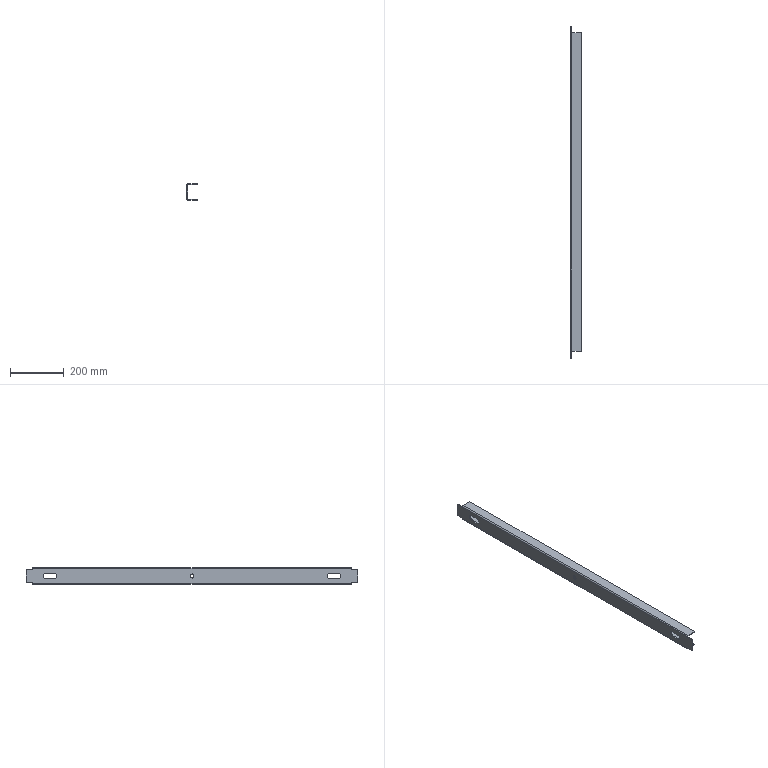Part | SolidWorks | features SMBaseFlange 2, Cut 1, Fillet 1, FlatPattern 1, SheetMetal 1 | 1 solid | 44 faces | box 40 x 1240 x 62 mm | volume 630088 mm3 | plane 30 | cylinder 14 | commonest cylinder face diameters 10 x4 20 x4 0.4 x2 8.4 x2 15 x2
STEP:
#1=CARTESIAN_POINT('',(0.,0.,-7.5));
#2=VERTEX_POINT('',#1);
#3=CARTESIAN_POINT('',(0.,0.,7.5));
#4=VERTEX_POINT('',#3);
#5=CARTESIAN_POINT('',(0.,0.,0.));
#6=DIRECTION('',(-1.,0.,0.));
#7=DIRECTION('',(0.,0.,1.));
#8=AXIS2_PLACEMENT_3D('',#5,#6,#7);
#9=CIRCLE('',#8,7.5);
#10=EDGE_CURVE('',#2,#4,#9,.T.);
#11=ORIENTED_EDGE('',*,*,#10,.T.);
#12=CARTESIAN_POINT('',(4.,0.,7.5));
#13=VERTEX_POINT('',#12);
#14=CARTESIAN_POINT('',(-6.,0.,7.5));
#15=DIRECTION('',(1.,0.,0.));
#16=VECTOR('',#15,1000.);
#17=LINE('',#14,#16);
#18=EDGE_CURVE('',#4,#13,#17,.T.);
#19=ORIENTED_EDGE('',*,*,#18,.T.);
#20=CARTESIAN_POINT('',(4.,0.,-7.5));
#21=VERTEX_POINT('',#20);
#22=CARTESIAN_POINT('',(4.,0.,0.));
#23=DIRECTION('',(1.,0.,0.));
#24=DIRECTION('',(0.,0.,-1.));
#25=AXIS2_PLACEMENT_3D('',#22,#23,#24);
#26=CIRCLE('',#25,7.5);
#27=EDGE_CURVE('',#13,#21,#26,.T.);
#28=ORIENTED_EDGE('',*,*,#27,.T.);
#29=CARTESIAN_POINT('',(-6.,0.,-7.5));
#30=DIRECTION('',(1.,0.,0.));
#31=VECTOR('',#30,1000.);
#32=LINE('',#29,#31);
#33=EDGE_CURVE('',#2,#21,#32,.T.);
#34=ORIENTED_EDGE('',*,*,#33,.F.);
#35=EDGE_LOOP('',(#11,#19,#28,#34));
#36=FACE_OUTER_BOUND('',#35,.T.);
#37=CARTESIAN_POINT('',(-6.,0.,0.));
#38=DIRECTION('',(1.,0.,0.));
#39=DIRECTION('',(0.,0.,-1.));
#40=AXIS2_PLACEMENT_3D('',#37,#38,#39);
#41=CYLINDRICAL_SURFACE('',#40,7.5);
#42=ADVANCED_FACE('',(#36),#41,.F.);
#43=CARTESIAN_POINT('',(4.,-594.,25.));
#44=VERTEX_POINT('',#43);
#45=CARTESIAN_POINT('',(0.,-594.,25.));
#46=VERTEX_POINT('',#45);
#47=CARTESIAN_POINT('',(4.2,-594.,25.));
#48=DIRECTION('',(-1.,0.,0.));
#49=VECTOR('',#48,1000.);
#50=LINE('',#47,#49);
#51=EDGE_CURVE('',#44,#46,#50,.T.);
#52=ORIENTED_EDGE('',*,*,#51,.F.);
#53=CARTESIAN_POINT('',(4.,-594.,26.8));
#54=VERTEX_POINT('',#53);
#55=CARTESIAN_POINT('',(4.,-594.,-31.));
#56=DIRECTION('',(0.,0.,-1.));
#57=VECTOR('',#56,1000.);
#58=LINE('',#55,#57);
#59=EDGE_CURVE('',#54,#44,#58,.T.);
#60=ORIENTED_EDGE('',*,*,#59,.F.);
#61=CARTESIAN_POINT('',(0.,-594.,26.8));
#62=VERTEX_POINT('',#61);
#63=CARTESIAN_POINT('',(4.,-594.,26.8));
#64=DIRECTION('',(-1.,0.,0.));
#65=VECTOR('',#64,1000.);
#66=LINE('',#63,#65);
#67=EDGE_CURVE('',#54,#62,#66,.T.);
#68=ORIENTED_EDGE('',*,*,#67,.T.);
#69=CARTESIAN_POINT('',(0.,-594.,-31.));
#70=DIRECTION('',(0.,0.,-1.));
#71=VECTOR('',#70,1000.);
#72=LINE('',#69,#71);
#73=EDGE_CURVE('',#62,#46,#72,.T.);
#74=ORIENTED_EDGE('',*,*,#73,.T.);
#75=EDGE_LOOP('',(#52,#60,#68,#74));
#76=FACE_OUTER_BOUND('',#75,.T.);
#77=CARTESIAN_POINT('',(4.2,-594.,-27.));
#78=DIRECTION('',(0.,-1.,0.));
#79=DIRECTION('',(0.,0.,-1.));
#80=AXIS2_PLACEMENT_3D('',#77,#78,#79);
#81=PLANE('',#80);
#82=ADVANCED_FACE('',(#76),#81,.T.);
#83=CARTESIAN_POINT('',(4.,594.,-25.));
#84=VERTEX_POINT('',#83);
#85=CARTESIAN_POINT('',(0.,594.,-25.));
#86=VERTEX_POINT('',#85);
#87=CARTESIAN_POINT('',(4.2,594.,-25.));
#88=DIRECTION('',(-1.,0.,0.));
#89=VECTOR('',#88,1000.);
#90=LINE('',#87,#89);
#91=EDGE_CURVE('',#84,#86,#90,.T.);
#92=ORIENTED_EDGE('',*,*,#91,.F.);
#93=CARTESIAN_POINT('',(4.,594.,-26.8));
#94=VERTEX_POINT('',#93);
#95=CARTESIAN_POINT('',(4.,594.,-31.));
#96=DIRECTION('',(0.,0.,-1.));
#97=VECTOR('',#96,1000.);
#98=LINE('',#95,#97);
#99=EDGE_CURVE('',#84,#94,#98,.T.);
#100=ORIENTED_EDGE('',*,*,#99,.T.);
#101=CARTESIAN_POINT('',(0.,594.,-26.8));
#102=VERTEX_POINT('',#101);
#103=CARTESIAN_POINT('',(4.,594.,-26.8));
#104=DIRECTION('',(-1.,0.,0.));
#105=VECTOR('',#104,1000.);
#106=LINE('',#103,#105);
#107=EDGE_CURVE('',#94,#102,#106,.T.);
#108=ORIENTED_EDGE('',*,*,#107,.T.);
#109=CARTESIAN_POINT('',(0.,594.,-31.));
#110=DIRECTION('',(0.,0.,-1.));
#111=VECTOR('',#110,1000.);
#112=LINE('',#109,#111);
#113=EDGE_CURVE('',#86,#102,#112,.T.);
#114=ORIENTED_EDGE('',*,*,#113,.F.);
#115=EDGE_LOOP('',(#92,#100,#108,#114));
#116=FACE_OUTER_BOUND('',#115,.T.);
#117=CARTESIAN_POINT('',(4.2,594.,27.));
#118=DIRECTION('',(0.,1.,0.));
#119=DIRECTION('',(0.,0.,1.));
#120=AXIS2_PLACEMENT_3D('',#117,#118,#119);
#121=PLANE('',#120);
#122=ADVANCED_FACE('',(#116),#121,.T.);
#123=CARTESIAN_POINT('',(0.,594.,26.8));
#124=VERTEX_POINT('',#123);
#125=CARTESIAN_POINT('',(4.,594.,26.8));
#126=VERTEX_POINT('',#125);
#127=CARTESIAN_POINT('',(0.,594.,26.8));
#128=DIRECTION('',(1.,0.,0.));
#129=VECTOR('',#128,1000.);
#130=LINE('',#127,#129);
#131=EDGE_CURVE('',#124,#126,#130,.T.);
#132=ORIENTED_EDGE('',*,*,#131,.F.);
#133=CARTESIAN_POINT('',(4.2,594.,31.));
#134=VERTEX_POINT('',#133);
#135=CARTESIAN_POINT('',(4.2,594.,26.8));
#136=DIRECTION('',(0.,-1.,0.));
#137=DIRECTION('',(0.,0.,1.));
#138=AXIS2_PLACEMENT_3D('',#135,#136,#137);
#139=CIRCLE('',#138,4.2);
#140=EDGE_CURVE('',#134,#124,#139,.T.);
#141=ORIENTED_EDGE('',*,*,#140,.F.);
#142=CARTESIAN_POINT('',(4.2,594.,27.));
#143=VERTEX_POINT('',#142);
#144=CARTESIAN_POINT('',(4.2,594.,27.));
#145=DIRECTION('',(0.,0.,1.));
#146=VECTOR('',#145,1000.);
#147=LINE('',#144,#146);
#148=EDGE_CURVE('',#143,#134,#147,.T.);
#149=ORIENTED_EDGE('',*,*,#148,.F.);
#150=CARTESIAN_POINT('',(4.2,594.,26.8));
#151=DIRECTION('',(0.,-1.,0.));
#152=DIRECTION('',(1.,0.,0.));
#153=AXIS2_PLACEMENT_3D('',#150,#151,#152);
#154=CIRCLE('',#153,0.2);
#155=EDGE_CURVE('',#143,#126,#154,.T.);
#156=ORIENTED_EDGE('',*,*,#155,.T.);
#157=EDGE_LOOP('',(#132,#141,#149,#156));
#158=FACE_OUTER_BOUND('',#157,.T.);
#159=CARTESIAN_POINT('',(0.,594.,26.8));
#160=DIRECTION('',(0.,1.,0.));
#161=DIRECTION('',(0.,0.,1.));
#162=AXIS2_PLACEMENT_3D('',#159,#160,#161);
#163=PLANE('',#162);
#164=ADVANCED_FACE('',(#158),#163,.T.);
#165=CARTESIAN_POINT('',(0.,594.,25.));
#166=VERTEX_POINT('',#165);
#167=CARTESIAN_POINT('',(4.,594.,25.));
#168=VERTEX_POINT('',#167);
#169=CARTESIAN_POINT('',(4.2,594.,25.));
#170=DIRECTION('',(1.,0.,0.));
#171=VECTOR('',#170,1000.);
#172=LINE('',#169,#171);
#173=EDGE_CURVE('',#166,#168,#172,.T.);
#174=ORIENTED_EDGE('',*,*,#173,.F.);
#175=CARTESIAN_POINT('',(0.,594.,-31.));
#176=DIRECTION('',(0.,0.,-1.));
#177=VECTOR('',#176,1000.);
#178=LINE('',#175,#177);
#179=EDGE_CURVE('',#124,#166,#178,.T.);
#180=ORIENTED_EDGE('',*,*,#179,.F.);
#181=ORIENTED_EDGE('',*,*,#131,.T.);
#182=CARTESIAN_POINT('',(4.,594.,-31.));
#183=DIRECTION('',(0.,0.,-1.));
#184=VECTOR('',#183,1000.);
#185=LINE('',#182,#184);
#186=EDGE_CURVE('',#126,#168,#185,.T.);
#187=ORIENTED_EDGE('',*,*,#186,.T.);
#188=EDGE_LOOP('',(#174,#180,#181,#187));
#189=FACE_OUTER_BOUND('',#188,.T.);
#190=CARTESIAN_POINT('',(4.2,594.,27.));
#191=DIRECTION('',(0.,1.,0.));
#192=DIRECTION('',(0.,0.,1.));
#193=AXIS2_PLACEMENT_3D('',#190,#191,#192);
#194=PLANE('',#193);
#195=ADVANCED_FACE('',(#189),#194,.T.);
#196=CARTESIAN_POINT('',(4.2,-594.,31.));
#197=VERTEX_POINT('',#196);
#198=CARTESIAN_POINT('',(4.2,-594.,27.));
#199=VERTEX_POINT('',#198);
#200=CARTESIAN_POINT('',(4.2,-594.,31.));
#201=DIRECTION('',(0.,0.,-1.));
#202=VECTOR('',#201,1000.);
#203=LINE('',#200,#202);
#204=EDGE_CURVE('',#197,#199,#203,.T.);
#205=ORIENTED_EDGE('',*,*,#204,.F.);
#206=CARTESIAN_POINT('',(4.2,-594.,26.8));
#207=DIRECTION('',(0.,-1.,0.));
#208=DIRECTION('',(0.,0.,1.));
#209=AXIS2_PLACEMENT_3D('',#206,#207,#208);
#210=CIRCLE('',#209,4.2);
#211=EDGE_CURVE('',#197,#62,#210,.T.);
#212=ORIENTED_EDGE('',*,*,#211,.T.);
#213=ORIENTED_EDGE('',*,*,#67,.F.);
#214=CARTESIAN_POINT('',(4.2,-594.,26.8));
#215=DIRECTION('',(0.,-1.,0.));
#216=DIRECTION('',(1.,0.,0.));
#217=AXIS2_PLACEMENT_3D('',#214,#215,#216);
#218=CIRCLE('',#217,0.2);
#219=EDGE_CURVE('',#199,#54,#218,.T.);
#220=ORIENTED_EDGE('',*,*,#219,.F.);
#221=EDGE_LOOP('',(#205,#212,#213,#220));
#222=FACE_OUTER_BOUND('',#221,.T.);
#223=CARTESIAN_POINT('',(4.2,-594.,31.));
#224=DIRECTION('',(0.,-1.,0.));
#225=DIRECTION('',(0.,0.,-1.));
#226=AXIS2_PLACEMENT_3D('',#223,#224,#225);
#227=PLANE('',#226);
#228=ADVANCED_FACE('',(#222),#227,.T.);
#229=CARTESIAN_POINT('',(40.,-594.,31.));
#230=VERTEX_POINT('',#229);
#231=CARTESIAN_POINT('',(0.,-594.,31.));
#232=DIRECTION('',(-1.,0.,0.));
#233=VECTOR('',#232,1000.);
#234=LINE('',#231,#233);
#235=EDGE_CURVE('',#230,#197,#234,.T.);
#236=ORIENTED_EDGE('',*,*,#235,.T.);
#237=ORIENTED_EDGE('',*,*,#204,.T.);
#238=CARTESIAN_POINT('',(40.,-594.,27.));
#239=VERTEX_POINT('',#238);
#240=CARTESIAN_POINT('',(0.,-594.,27.));
#241=DIRECTION('',(-1.,0.,0.));
#242=VECTOR('',#241,1000.);
#243=LINE('',#240,#242);
#244=EDGE_CURVE('',#239,#199,#243,.T.);
#245=ORIENTED_EDGE('',*,*,#244,.F.);
#246=CARTESIAN_POINT('',(40.,-594.,27.));
#247=DIRECTION('',(0.,0.,1.));
#248=VECTOR('',#247,1000.);
#249=LINE('',#246,#248);
#250=EDGE_CURVE('',#239,#230,#249,.T.);
#251=ORIENTED_EDGE('',*,*,#250,.T.);
#252=EDGE_LOOP('',(#236,#237,#245,#251));
#253=FACE_OUTER_BOUND('',#252,.T.);
#254=CARTESIAN_POINT('',(4.,-594.,26.8));
#255=DIRECTION('',(0.,-1.,0.));
#256=DIRECTION('',(0.,0.,-1.));
#257=AXIS2_PLACEMENT_3D('',#254,#255,#256);
#258=PLANE('',#257);
#259=ADVANCED_FACE('',(#253),#258,.T.);
#260=CARTESIAN_POINT('',(4.2,594.,-31.));
#261=VERTEX_POINT('',#260);
#262=CARTESIAN_POINT('',(4.2,594.,-27.));
#263=VERTEX_POINT('',#262);
#264=CARTESIAN_POINT('',(4.2,594.,-31.));
#265=DIRECTION('',(0.,0.,1.));
#266=VECTOR('',#265,1000.);
#267=LINE('',#264,#266);
#268=EDGE_CURVE('',#261,#263,#267,.T.);
#269=ORIENTED_EDGE('',*,*,#268,.F.);
#270=CARTESIAN_POINT('',(4.2,594.,-26.8));
#271=DIRECTION('',(0.,-1.,0.));
#272=DIRECTION('',(0.,0.,1.));
#273=AXIS2_PLACEMENT_3D('',#270,#271,#272);
#274=CIRCLE('',#273,4.2);
#275=EDGE_CURVE('',#102,#261,#274,.T.);
#276=ORIENTED_EDGE('',*,*,#275,.F.);
#277=ORIENTED_EDGE('',*,*,#107,.F.);
#278=CARTESIAN_POINT('',(4.2,594.,-26.8));
#279=DIRECTION('',(0.,-1.,0.));
#280=DIRECTION('',(1.,0.,0.));
#281=AXIS2_PLACEMENT_3D('',#278,#279,#280);
#282=CIRCLE('',#281,0.2);
#283=EDGE_CURVE('',#94,#263,#282,.T.);
#284=ORIENTED_EDGE('',*,*,#283,.T.);
#285=EDGE_LOOP('',(#269,#276,#277,#284));
#286=FACE_OUTER_BOUND('',#285,.T.);
#287=CARTESIAN_POINT('',(4.2,594.,-31.));
#288=DIRECTION('',(0.,1.,0.));
#289=DIRECTION('',(0.,0.,1.));
#290=AXIS2_PLACEMENT_3D('',#287,#288,#289);
#291=PLANE('',#290);
#292=ADVANCED_FACE('',(#286),#291,.T.);
#293=CARTESIAN_POINT('',(40.,594.,-31.));
#294=VERTEX_POINT('',#293);
#295=CARTESIAN_POINT('',(0.,594.,-31.));
#296=DIRECTION('',(1.,0.,0.));
#297=VECTOR('',#296,1000.);
#298=LINE('',#295,#297);
#299=EDGE_CURVE('',#261,#294,#298,.T.);
#300=ORIENTED_EDGE('',*,*,#299,.F.);
#301=ORIENTED_EDGE('',*,*,#268,.T.);
#302=CARTESIAN_POINT('',(40.,594.,-27.));
#303=VERTEX_POINT('',#302);
#304=CARTESIAN_POINT('',(0.,594.,-27.));
#305=DIRECTION('',(1.,0.,0.));
#306=VECTOR('',#305,1000.);
#307=LINE('',#304,#306);
#308=EDGE_CURVE('',#263,#303,#307,.T.);
#309=ORIENTED_EDGE('',*,*,#308,.T.);
#310=CARTESIAN_POINT('',(40.,594.,-31.));
#311=DIRECTION('',(0.,0.,1.));
#312=VECTOR('',#311,1000.);
#313=LINE('',#310,#312);
#314=EDGE_CURVE('',#294,#303,#313,.T.);
#315=ORIENTED_EDGE('',*,*,#314,.F.);
#316=EDGE_LOOP('',(#300,#301,#309,#315));
#317=FACE_OUTER_BOUND('',#316,.T.);
#318=CARTESIAN_POINT('',(4.,594.,-26.8));
#319=DIRECTION('',(0.,1.,0.));
#320=DIRECTION('',(0.,0.,1.));
#321=AXIS2_PLACEMENT_3D('',#318,#319,#320);
#322=PLANE('',#321);
#323=ADVANCED_FACE('',(#317),#322,.T.);
#324=CARTESIAN_POINT('',(0.,-594.,-26.8));
#325=VERTEX_POINT('',#324);
#326=CARTESIAN_POINT('',(4.,-594.,-26.8));
#327=VERTEX_POINT('',#326);
#328=CARTESIAN_POINT('',(0.,-594.,-26.8));
#329=DIRECTION('',(1.,0.,0.));
#330=VECTOR('',#329,1000.);
#331=LINE('',#328,#330);
#332=EDGE_CURVE('',#325,#327,#331,.T.);
#333=ORIENTED_EDGE('',*,*,#332,.F.);
#334=CARTESIAN_POINT('',(4.2,-594.,-31.));
#335=VERTEX_POINT('',#334);
#336=CARTESIAN_POINT('',(4.2,-594.,-26.8));
#337=DIRECTION('',(0.,-1.,0.));
#338=DIRECTION('',(0.,0.,1.));
#339=AXIS2_PLACEMENT_3D('',#336,#337,#338);
#340=CIRCLE('',#339,4.2);
#341=EDGE_CURVE('',#325,#335,#340,.T.);
#342=ORIENTED_EDGE('',*,*,#341,.T.);
#343=CARTESIAN_POINT('',(4.2,-594.,-27.));
#344=VERTEX_POINT('',#343);
#345=CARTESIAN_POINT('',(4.2,-594.,-27.));
#346=DIRECTION('',(0.,0.,-1.));
#347=VECTOR('',#346,1000.);
#348=LINE('',#345,#347);
#349=EDGE_CURVE('',#344,#335,#348,.T.);
#350=ORIENTED_EDGE('',*,*,#349,.F.);
#351=CARTESIAN_POINT('',(4.2,-594.,-26.8));
#352=DIRECTION('',(0.,-1.,0.));
#353=DIRECTION('',(1.,0.,0.));
#354=AXIS2_PLACEMENT_3D('',#351,#352,#353);
#355=CIRCLE('',#354,0.2);
#356=EDGE_CURVE('',#327,#344,#355,.T.);
#357=ORIENTED_EDGE('',*,*,#356,.F.);
#358=EDGE_LOOP('',(#333,#342,#350,#357));
#359=FACE_OUTER_BOUND('',#358,.T.);
#360=CARTESIAN_POINT('',(0.,-594.,-26.8));
#361=DIRECTION('',(0.,-1.,0.));
#362=DIRECTION('',(0.,0.,-1.));
#363=AXIS2_PLACEMENT_3D('',#360,#361,#362);
#364=PLANE('',#363);
#365=ADVANCED_FACE('',(#359),#364,.T.);
#366=CARTESIAN_POINT('',(0.,-594.,-25.));
#367=VERTEX_POINT('',#366);
#368=CARTESIAN_POINT('',(4.,-594.,-25.));
#369=VERTEX_POINT('',#368);
#370=CARTESIAN_POINT('',(4.2,-594.,-25.));
#371=DIRECTION('',(1.,0.,0.));
#372=VECTOR('',#371,1000.);
#373=LINE('',#370,#372);
#374=EDGE_CURVE('',#367,#369,#373,.T.);
#375=ORIENTED_EDGE('',*,*,#374,.F.);
#376=CARTESIAN_POINT('',(0.,-594.,-31.));
#377=DIRECTION('',(0.,0.,-1.));
#378=VECTOR('',#377,1000.);
#379=LINE('',#376,#378);
#380=EDGE_CURVE('',#367,#325,#379,.T.);
#381=ORIENTED_EDGE('',*,*,#380,.T.);
#382=ORIENTED_EDGE('',*,*,#332,.T.);
#383=CARTESIAN_POINT('',(4.,-594.,-31.));
#384=DIRECTION('',(0.,0.,-1.));
#385=VECTOR('',#384,1000.);
#386=LINE('',#383,#385);
#387=EDGE_CURVE('',#369,#327,#386,.T.);
#388=ORIENTED_EDGE('',*,*,#387,.F.);
#389=EDGE_LOOP('',(#375,#381,#382,#388));
#390=FACE_OUTER_BOUND('',#389,.T.);
#391=CARTESIAN_POINT('',(4.2,-594.,-27.));
#392=DIRECTION('',(0.,-1.,0.));
#393=DIRECTION('',(0.,0.,-1.));
#394=AXIS2_PLACEMENT_3D('',#391,#392,#393);
#395=PLANE('',#394);
#396=ADVANCED_FACE('',(#390),#395,.T.);
#397=CARTESIAN_POINT('',(40.,-594.,-27.));
#398=VERTEX_POINT('',#397);
#399=CARTESIAN_POINT('',(0.,-594.,-27.));
#400=DIRECTION('',(1.,0.,0.));
#401=VECTOR('',#400,1000.);
#402=LINE('',#399,#401);
#403=EDGE_CURVE('',#344,#398,#402,.T.);
#404=ORIENTED_EDGE('',*,*,#403,.T.);
#405=CARTESIAN_POINT('',(40.,594.,-27.));
#406=DIRECTION('',(0.,-1.,0.));
#407=VECTOR('',#406,1000.);
#408=LINE('',#405,#407);
#409=EDGE_CURVE('',#303,#398,#408,.T.);
#410=ORIENTED_EDGE('',*,*,#409,.F.);
#411=ORIENTED_EDGE('',*,*,#308,.F.);
#412=CARTESIAN_POINT('',(4.2,594.,-27.));
#413=DIRECTION('',(0.,-1.,0.));
#414=VECTOR('',#413,1000.);
#415=LINE('',#412,#414);
#416=EDGE_CURVE('',#263,#344,#415,.T.);
#417=ORIENTED_EDGE('',*,*,#416,.T.);
#418=EDGE_LOOP('',(#404,#410,#411,#417));
#419=FACE_OUTER_BOUND('',#418,.T.);
#420=CARTESIAN_POINT('',(0.,594.,-27.));
#421=DIRECTION('',(0.,0.,-1.));
#422=DIRECTION('',(-1.,0.,0.));
#423=AXIS2_PLACEMENT_3D('',#420,#421,#422);
#424=PLANE('',#423);
#425=ADVANCED_FACE('',(#419),#424,.F.);
#426=CARTESIAN_POINT('',(40.,-594.,-31.));
#427=VERTEX_POINT('',#426);
#428=CARTESIAN_POINT('',(40.,-594.,-31.));
#429=DIRECTION('',(0.,0.,1.));
#430=VECTOR('',#429,1000.);
#431=LINE('',#428,#430);
#432=EDGE_CURVE('',#427,#398,#431,.T.);
#433=ORIENTED_EDGE('',*,*,#432,.F.);
#434=CARTESIAN_POINT('',(40.,594.,-31.));
#435=DIRECTION('',(0.,-1.,0.));
#436=VECTOR('',#435,1000.);
#437=LINE('',#434,#436);
#438=EDGE_CURVE('',#294,#427,#437,.T.);
#439=ORIENTED_EDGE('',*,*,#438,.F.);
#440=ORIENTED_EDGE('',*,*,#314,.T.);
#441=ORIENTED_EDGE('',*,*,#409,.T.);
#442=EDGE_LOOP('',(#433,#439,#440,#441));
#443=FACE_OUTER_BOUND('',#442,.T.);
#444=CARTESIAN_POINT('',(40.,594.,-31.));
#445=DIRECTION('',(1.,0.,0.));
#446=DIRECTION('',(0.,0.,-1.));
#447=AXIS2_PLACEMENT_3D('',#444,#445,#446);
#448=PLANE('',#447);
#449=ADVANCED_FACE('',(#443),#448,.T.);
#450=CARTESIAN_POINT('',(0.,-594.,-31.));
#451=DIRECTION('',(1.,0.,0.));
#452=VECTOR('',#451,1000.);
#453=LINE('',#450,#452);
#454=EDGE_CURVE('',#335,#427,#453,.T.);
#455=ORIENTED_EDGE('',*,*,#454,.F.);
#456=CARTESIAN_POINT('',(4.2,594.,-31.));
#457=DIRECTION('',(0.,-1.,0.));
#458=VECTOR('',#457,1000.);
#459=LINE('',#456,#458);
#460=EDGE_CURVE('',#261,#335,#459,.T.);
#461=ORIENTED_EDGE('',*,*,#460,.F.);
#462=ORIENTED_EDGE('',*,*,#299,.T.);
#463=ORIENTED_EDGE('',*,*,#438,.T.);
#464=EDGE_LOOP('',(#455,#461,#462,#463));
#465=FACE_OUTER_BOUND('',#464,.T.);
#466=CARTESIAN_POINT('',(0.,594.,-31.));
#467=DIRECTION('',(0.,0.,-1.));
#468=DIRECTION('',(-1.,0.,0.));
#469=AXIS2_PLACEMENT_3D('',#466,#467,#468);
#470=PLANE('',#469);
#471=ADVANCED_FACE('',(#465),#470,.T.);
#472=ORIENTED_EDGE('',*,*,#341,.F.);
#473=CARTESIAN_POINT('',(0.,594.,-26.8));
#474=DIRECTION('',(0.,-1.,0.));
#475=VECTOR('',#474,1000.);
#476=LINE('',#473,#475);
#477=EDGE_CURVE('',#102,#325,#476,.T.);
#478=ORIENTED_EDGE('',*,*,#477,.F.);
#479=ORIENTED_EDGE('',*,*,#275,.T.);
#480=ORIENTED_EDGE('',*,*,#460,.T.);
#481=EDGE_LOOP('',(#472,#478,#479,#480));
#482=FACE_OUTER_BOUND('',#481,.T.);
#483=CARTESIAN_POINT('',(4.2,594.,-26.8));
#484=DIRECTION('',(0.,-1.,0.));
#485=DIRECTION('',(0.,0.,-1.));
#486=AXIS2_PLACEMENT_3D('',#483,#484,#485);
#487=CYLINDRICAL_SURFACE('',#486,4.2);
#488=ADVANCED_FACE('',(#482),#487,.T.);
#489=CARTESIAN_POINT('',(0.,515.,-10.));
#490=VERTEX_POINT('',#489);
#491=CARTESIAN_POINT('',(0.,515.,10.));
#492=VERTEX_POINT('',#491);
#493=CARTESIAN_POINT('',(0.,515.,0.));
#494=DIRECTION('',(-1.,0.,0.));
#495=DIRECTION('',(0.,0.,1.));
#496=AXIS2_PLACEMENT_3D('',#493,#494,#495);
#497=CIRCLE('',#496,10.);
#498=EDGE_CURVE('',#490,#492,#497,.T.);
#499=ORIENTED_EDGE('',*,*,#498,.F.);
#500=CARTESIAN_POINT('',(0.,545.,-10.));
#501=VERTEX_POINT('',#500);
#502=CARTESIAN_POINT('',(0.,594.,-10.));
#503=DIRECTION('',(0.,-1.,0.));
#504=VECTOR('',#503,1000.);
#505=LINE('',#502,#504);
#506=EDGE_CURVE('',#501,#490,#505,.T.);
#507=ORIENTED_EDGE('',*,*,#506,.F.);
#508=CARTESIAN_POINT('',(0.,545.,10.));
#509=VERTEX_POINT('',#508);
#510=CARTESIAN_POINT('',(0.,545.,0.));
#511=DIRECTION('',(-1.,0.,0.));
#512=DIRECTION('',(0.,0.,1.));
#513=AXIS2_PLACEMENT_3D('',#510,#511,#512);
#514=CIRCLE('',#513,10.);
#515=EDGE_CURVE('',#509,#501,#514,.T.);
#516=ORIENTED_EDGE('',*,*,#515,.F.);
#517=CARTESIAN_POINT('',(0.,594.,10.));
#518=DIRECTION('',(0.,1.,0.));
#519=VECTOR('',#518,1000.);
#520=LINE('',#517,#519);
#521=EDGE_CURVE('',#492,#509,#520,.T.);
#522=ORIENTED_EDGE('',*,*,#521,.F.);
#523=EDGE_LOOP('',(#499,#507,#516,#522));
#524=FACE_BOUND('',#523,.T.);
#525=ORIENTED_EDGE('',*,*,#10,.F.);
#526=CARTESIAN_POINT('',(0.,0.,0.));
#527=DIRECTION('',(-1.,0.,0.));
#528=DIRECTION('',(0.,0.,1.));
#529=AXIS2_PLACEMENT_3D('',#526,#527,#528);
#530=CIRCLE('',#529,7.5);
#531=EDGE_CURVE('',#4,#2,#530,.T.);
#532=ORIENTED_EDGE('',*,*,#531,.F.);
#533=EDGE_LOOP('',(#525,#532));
#534=FACE_BOUND('',#533,.T.);
#535=CARTESIAN_POINT('',(0.,-515.,10.));
#536=VERTEX_POINT('',#535);
#537=CARTESIAN_POINT('',(0.,-515.,-10.));
#538=VERTEX_POINT('',#537);
#539=CARTESIAN_POINT('',(0.,-515.,0.));
#540=DIRECTION('',(-1.,0.,0.));
#541=DIRECTION('',(0.,0.,1.));
#542=AXIS2_PLACEMENT_3D('',#539,#540,#541);
#543=CIRCLE('',#542,10.);
#544=EDGE_CURVE('',#536,#538,#543,.T.);
#545=ORIENTED_EDGE('',*,*,#544,.F.);
#546=CARTESIAN_POINT('',(0.,-545.,10.));
#547=VERTEX_POINT('',#546);
#548=CARTESIAN_POINT('',(0.,594.,10.));
#549=DIRECTION('',(0.,1.,0.));
#550=VECTOR('',#549,1000.);
#551=LINE('',#548,#550);
#552=EDGE_CURVE('',#547,#536,#551,.T.);
#553=ORIENTED_EDGE('',*,*,#552,.F.);
#554=CARTESIAN_POINT('',(0.,-545.,-10.));
#555=VERTEX_POINT('',#554);
#556=CARTESIAN_POINT('',(0.,-545.,0.));
#557=DIRECTION('',(-1.,0.,0.));
#558=DIRECTION('',(0.,0.,1.));
#559=AXIS2_PLACEMENT_3D('',#556,#557,#558);
#560=CIRCLE('',#559,10.);
#561=EDGE_CURVE('',#555,#547,#560,.T.);
#562=ORIENTED_EDGE('',*,*,#561,.F.);
#563=CARTESIAN_POINT('',(0.,594.,-10.));
#564=DIRECTION('',(0.,-1.,0.));
#565=VECTOR('',#564,1000.);
#566=LINE('',#563,#565);
#567=EDGE_CURVE('',#538,#555,#566,.T.);
#568=ORIENTED_EDGE('',*,*,#567,.F.);
#569=EDGE_LOOP('',(#545,#553,#562,#568));
#570=FACE_BOUND('',#569,.T.);
#571=CARTESIAN_POINT('',(0.,-615.,-25.));
#572=VERTEX_POINT('',#571);
#573=CARTESIAN_POINT('',(0.,-620.,-25.));
#574=DIRECTION('',(0.,1.,0.));
#575=VECTOR('',#574,1000.);
#576=LINE('',#573,#575);
#577=EDGE_CURVE('',#572,#367,#576,.T.);
#578=ORIENTED_EDGE('',*,*,#577,.F.);
#579=CARTESIAN_POINT('',(0.,-620.,-20.));
#580=VERTEX_POINT('',#579);
#581=CARTESIAN_POINT('',(0.,-615.,-20.));
#582=DIRECTION('',(-1.,0.,0.));
#583=DIRECTION('',(0.,0.,1.));
#584=AXIS2_PLACEMENT_3D('',#581,#582,#583);
#585=CIRCLE('',#584,5.);
#586=EDGE_CURVE('',#572,#580,#585,.T.);
#587=ORIENTED_EDGE('',*,*,#586,.T.);
#588=CARTESIAN_POINT('',(0.,-620.,20.));
#589=VERTEX_POINT('',#588);
#590=CARTESIAN_POINT('',(0.,-620.,25.));
#591=DIRECTION('',(0.,0.,-1.));
#592=VECTOR('',#591,1000.);
#593=LINE('',#590,#592);
#594=EDGE_CURVE('',#589,#580,#593,.T.);
#595=ORIENTED_EDGE('',*,*,#594,.F.);
#596=CARTESIAN_POINT('',(0.,-615.,25.));
#597=VERTEX_POINT('',#596);
#598=CARTESIAN_POINT('',(0.,-615.,20.));
#599=DIRECTION('',(-1.,0.,0.));
#600=DIRECTION('',(0.,0.,1.));
#601=AXIS2_PLACEMENT_3D('',#598,#599,#600);
#602=CIRCLE('',#601,5.);
#603=EDGE_CURVE('',#589,#597,#602,.T.);
#604=ORIENTED_EDGE('',*,*,#603,.T.);
#605=CARTESIAN_POINT('',(0.,-620.,25.));
#606=DIRECTION('',(0.,-1.,0.));
#607=VECTOR('',#606,1000.);
#608=LINE('',#605,#607);
#609=EDGE_CURVE('',#46,#597,#608,.T.);
#610=ORIENTED_EDGE('',*,*,#609,.F.);
#611=ORIENTED_EDGE('',*,*,#73,.F.);
#612=CARTESIAN_POINT('',(0.,594.,26.8));
#613=DIRECTION('',(0.,-1.,0.));
#614=VECTOR('',#613,1000.);
#615=LINE('',#612,#614);
#616=EDGE_CURVE('',#124,#62,#615,.T.);
#617=ORIENTED_EDGE('',*,*,#616,.F.);
#618=ORIENTED_EDGE('',*,*,#179,.T.);
#619=CARTESIAN_POINT('',(0.,615.,25.));
#620=VERTEX_POINT('',#619);
#621=CARTESIAN_POINT('',(0.,620.,25.));
#622=DIRECTION('',(0.,-1.,0.));
#623=VECTOR('',#622,1000.);
#624=LINE('',#621,#623);
#625=EDGE_CURVE('',#620,#166,#624,.T.);
#626=ORIENTED_EDGE('',*,*,#625,.F.);
#627=CARTESIAN_POINT('',(0.,620.,20.));
#628=VERTEX_POINT('',#627);
#629=CARTESIAN_POINT('',(0.,615.,20.));
#630=DIRECTION('',(-1.,0.,0.));
#631=DIRECTION('',(0.,0.,1.));
#632=AXIS2_PLACEMENT_3D('',#629,#630,#631);
#633=CIRCLE('',#632,5.);
#634=EDGE_CURVE('',#620,#628,#633,.T.);
#635=ORIENTED_EDGE('',*,*,#634,.T.);
#636=CARTESIAN_POINT('',(0.,620.,-20.));
#637=VERTEX_POINT('',#636);
#638=CARTESIAN_POINT('',(0.,620.,25.));
#639=DIRECTION('',(0.,0.,1.));
#640=VECTOR('',#639,1000.);
#641=LINE('',#638,#640);
#642=EDGE_CURVE('',#637,#628,#641,.T.);
#643=ORIENTED_EDGE('',*,*,#642,.F.);
#644=CARTESIAN_POINT('',(0.,615.,-25.));
#645=VERTEX_POINT('',#644);
#646=CARTESIAN_POINT('',(0.,615.,-20.));
#647=DIRECTION('',(-1.,0.,0.));
#648=DIRECTION('',(0.,0.,1.));
#649=AXIS2_PLACEMENT_3D('',#646,#647,#648);
#650=CIRCLE('',#649,5.);
#651=EDGE_CURVE('',#637,#645,#650,.T.);
#652=ORIENTED_EDGE('',*,*,#651,.T.);
#653=CARTESIAN_POINT('',(0.,620.,-25.));
#654=DIRECTION('',(0.,1.,0.));
#655=VECTOR('',#654,1000.);
#656=LINE('',#653,#655);
#657=EDGE_CURVE('',#86,#645,#656,.T.);
#658=ORIENTED_EDGE('',*,*,#657,.F.);
#659=ORIENTED_EDGE('',*,*,#113,.T.);
#660=ORIENTED_EDGE('',*,*,#477,.T.);
#661=ORIENTED_EDGE('',*,*,#380,.F.);
#662=EDGE_LOOP('',(#578,#587,#595,#604,#610,#611,#617,#618,#626,#635,#643,#652,#658,#659,#660,#661));
#663=FACE_OUTER_BOUND('',#662,.T.);
#664=CARTESIAN_POINT('',(0.,594.,-31.));
#665=DIRECTION('',(-1.,0.,0.));
#666=DIRECTION('',(0.,0.,1.));
#667=AXIS2_PLACEMENT_3D('',#664,#665,#666);
#668=PLANE('',#667);
#669=ADVANCED_FACE('',(#524,#534,#570,#663),#668,.T.);
#670=ORIENTED_EDGE('',*,*,#211,.F.);
#671=CARTESIAN_POINT('',(4.2,594.,31.));
#672=DIRECTION('',(0.,-1.,0.));
#673=VECTOR('',#672,1000.);
#674=LINE('',#671,#673);
#675=EDGE_CURVE('',#134,#197,#674,.T.);
#676=ORIENTED_EDGE('',*,*,#675,.F.);
#677=ORIENTED_EDGE('',*,*,#140,.T.);
#678=ORIENTED_EDGE('',*,*,#616,.T.);
#679=EDGE_LOOP('',(#670,#676,#677,#678));
#680=FACE_OUTER_BOUND('',#679,.T.);
#681=CARTESIAN_POINT('',(4.2,594.,26.8));
#682=DIRECTION('',(0.,-1.,0.));
#683=DIRECTION('',(0.,0.,-1.));
#684=AXIS2_PLACEMENT_3D('',#681,#682,#683);
#685=CYLINDRICAL_SURFACE('',#684,4.2);
#686=ADVANCED_FACE('',(#680),#685,.T.);
#687=ORIENTED_EDGE('',*,*,#235,.F.);
#688=CARTESIAN_POINT('',(40.,594.,31.));
#689=VERTEX_POINT('',#688);
#690=CARTESIAN_POINT('',(40.,594.,31.));
#691=DIRECTION('',(0.,-1.,0.));
#692=VECTOR('',#691,1000.);
#693=LINE('',#690,#692);
#694=EDGE_CURVE('',#689,#230,#693,.T.);
#695=ORIENTED_EDGE('',*,*,#694,.F.);
#696=CARTESIAN_POINT('',(0.,594.,31.));
#697=DIRECTION('',(-1.,0.,0.));
#698=VECTOR('',#697,1000.);
#699=LINE('',#696,#698);
#700=EDGE_CURVE('',#689,#134,#699,.T.);
#701=ORIENTED_EDGE('',*,*,#700,.T.);
#702=ORIENTED_EDGE('',*,*,#675,.T.);
#703=EDGE_LOOP('',(#687,#695,#701,#702));
#704=FACE_OUTER_BOUND('',#703,.T.);
#705=CARTESIAN_POINT('',(0.,594.,31.));
#706=DIRECTION('',(0.,0.,1.));
#707=DIRECTION('',(1.,0.,0.));
#708=AXIS2_PLACEMENT_3D('',#705,#706,#707);
#709=PLANE('',#708);
#710=ADVANCED_FACE('',(#704),#709,.T.);
#711=ORIENTED_EDGE('',*,*,#250,.F.);
#712=CARTESIAN_POINT('',(40.,594.,27.));
#713=VERTEX_POINT('',#712);
#714=CARTESIAN_POINT('',(40.,594.,27.));
#715=DIRECTION('',(0.,-1.,0.));
#716=VECTOR('',#715,1000.);
#717=LINE('',#714,#716);
#718=EDGE_CURVE('',#713,#239,#717,.T.);
#719=ORIENTED_EDGE('',*,*,#718,.F.);
#720=CARTESIAN_POINT('',(40.,594.,27.));
#721=DIRECTION('',(0.,0.,1.));
#722=VECTOR('',#721,1000.);
#723=LINE('',#720,#722);
#724=EDGE_CURVE('',#713,#689,#723,.T.);
#725=ORIENTED_EDGE('',*,*,#724,.T.);
#726=ORIENTED_EDGE('',*,*,#694,.T.);
#727=EDGE_LOOP('',(#711,#719,#725,#726));
#728=FACE_OUTER_BOUND('',#727,.T.);
#729=CARTESIAN_POINT('',(40.,594.,27.));
#730=DIRECTION('',(1.,0.,0.));
#731=DIRECTION('',(0.,0.,-1.));
#732=AXIS2_PLACEMENT_3D('',#729,#730,#731);
#733=PLANE('',#732);
#734=ADVANCED_FACE('',(#728),#733,.T.);
#735=ORIENTED_EDGE('',*,*,#244,.T.);
#736=CARTESIAN_POINT('',(4.2,594.,27.));
#737=DIRECTION('',(0.,-1.,0.));
#738=VECTOR('',#737,1000.);
#739=LINE('',#736,#738);
#740=EDGE_CURVE('',#143,#199,#739,.T.);
#741=ORIENTED_EDGE('',*,*,#740,.F.);
#742=CARTESIAN_POINT('',(0.,594.,27.));
#743=DIRECTION('',(-1.,0.,0.));
#744=VECTOR('',#743,1000.);
#745=LINE('',#742,#744);
#746=EDGE_CURVE('',#713,#143,#745,.T.);
#747=ORIENTED_EDGE('',*,*,#746,.F.);
#748=ORIENTED_EDGE('',*,*,#718,.T.);
#749=EDGE_LOOP('',(#735,#741,#747,#748));
#750=FACE_OUTER_BOUND('',#749,.T.);
#751=CARTESIAN_POINT('',(0.,594.,27.));
#752=DIRECTION('',(0.,0.,1.));
#753=DIRECTION('',(1.,0.,0.));
#754=AXIS2_PLACEMENT_3D('',#751,#752,#753);
#755=PLANE('',#754);
#756=ADVANCED_FACE('',(#750),#755,.F.);
#757=ORIENTED_EDGE('',*,*,#219,.T.);
#758=CARTESIAN_POINT('',(4.,594.,26.8));
#759=DIRECTION('',(0.,-1.,0.));
#760=VECTOR('',#759,1000.);
#761=LINE('',#758,#760);
#762=EDGE_CURVE('',#126,#54,#761,.T.);
#763=ORIENTED_EDGE('',*,*,#762,.F.);
#764=ORIENTED_EDGE('',*,*,#155,.F.);
#765=ORIENTED_EDGE('',*,*,#740,.T.);
#766=EDGE_LOOP('',(#757,#763,#764,#765));
#767=FACE_OUTER_BOUND('',#766,.T.);
#768=CARTESIAN_POINT('',(4.2,594.,26.8));
#769=DIRECTION('',(0.,-1.,0.));
#770=DIRECTION('',(0.,0.,-1.));
#771=AXIS2_PLACEMENT_3D('',#768,#769,#770);
#772=CYLINDRICAL_SURFACE('',#771,0.2);
#773=ADVANCED_FACE('',(#767),#772,.F.);
#774=CARTESIAN_POINT('',(4.,515.,-10.));
#775=VERTEX_POINT('',#774);
#776=CARTESIAN_POINT('',(4.,545.,-10.));
#777=VERTEX_POINT('',#776);
#778=CARTESIAN_POINT('',(4.,515.,-10.));
#779=DIRECTION('',(0.,1.,0.));
#780=VECTOR('',#779,1000.);
#781=LINE('',#778,#780);
#782=EDGE_CURVE('',#775,#777,#781,.T.);
#783=ORIENTED_EDGE('',*,*,#782,.F.);
#784=CARTESIAN_POINT('',(4.,515.,10.));
#785=VERTEX_POINT('',#784);
#786=CARTESIAN_POINT('',(4.,515.,0.));
#787=DIRECTION('',(1.,0.,0.));
#788=DIRECTION('',(0.,0.,-1.));
#789=AXIS2_PLACEMENT_3D('',#786,#787,#788);
#790=CIRCLE('',#789,10.);
#791=EDGE_CURVE('',#785,#775,#790,.T.);
#792=ORIENTED_EDGE('',*,*,#791,.F.);
#793=CARTESIAN_POINT('',(4.,545.,10.));
#794=VERTEX_POINT('',#793);
#795=CARTESIAN_POINT('',(4.,515.,10.));
#796=DIRECTION('',(0.,-1.,0.));
#797=VECTOR('',#796,1000.);
#798=LINE('',#795,#797);
#799=EDGE_CURVE('',#794,#785,#798,.T.);
#800=ORIENTED_EDGE('',*,*,#799,.F.);
#801=CARTESIAN_POINT('',(4.,545.,0.));
#802=DIRECTION('',(1.,0.,0.));
#803=DIRECTION('',(0.,0.,-1.));
#804=AXIS2_PLACEMENT_3D('',#801,#802,#803);
#805=CIRCLE('',#804,10.);
#806=EDGE_CURVE('',#777,#794,#805,.T.);
#807=ORIENTED_EDGE('',*,*,#806,.F.);
#808=EDGE_LOOP('',(#783,#792,#800,#807));
#809=FACE_BOUND('',#808,.T.);
#810=CARTESIAN_POINT('',(4.,0.,0.));
#811=DIRECTION('',(1.,0.,0.));
#812=DIRECTION('',(0.,0.,-1.));
#813=AXIS2_PLACEMENT_3D('',#810,#811,#812);
#814=CIRCLE('',#813,7.5);
#815=EDGE_CURVE('',#21,#13,#814,.T.);
#816=ORIENTED_EDGE('',*,*,#815,.F.);
#817=ORIENTED_EDGE('',*,*,#27,.F.);
#818=EDGE_LOOP('',(#816,#817));
#819=FACE_BOUND('',#818,.T.);
#820=CARTESIAN_POINT('',(4.,-515.,10.));
#821=VERTEX_POINT('',#820);
#822=CARTESIAN_POINT('',(4.,-545.,10.));
#823=VERTEX_POINT('',#822);
#824=CARTESIAN_POINT('',(4.,-515.,10.));
#825=DIRECTION('',(0.,-1.,0.));
#826=VECTOR('',#825,1000.);
#827=LINE('',#824,#826);
#828=EDGE_CURVE('',#821,#823,#827,.T.);
#829=ORIENTED_EDGE('',*,*,#828,.F.);
#830=CARTESIAN_POINT('',(4.,-515.,-10.));
#831=VERTEX_POINT('',#830);
#832=CARTESIAN_POINT('',(4.,-515.,0.));
#833=DIRECTION('',(1.,0.,0.));
#834=DIRECTION('',(0.,0.,1.));
#835=AXIS2_PLACEMENT_3D('',#832,#833,#834);
#836=CIRCLE('',#835,10.);
#837=EDGE_CURVE('',#831,#821,#836,.T.);
#838=ORIENTED_EDGE('',*,*,#837,.F.);
#839=CARTESIAN_POINT('',(4.,-545.,-10.));
#840=VERTEX_POINT('',#839);
#841=CARTESIAN_POINT('',(4.,-515.,-10.));
#842=DIRECTION('',(0.,1.,0.));
#843=VECTOR('',#842,1000.);
#844=LINE('',#841,#843);
#845=EDGE_CURVE('',#840,#831,#844,.T.);
#846=ORIENTED_EDGE('',*,*,#845,.F.);
#847=CARTESIAN_POINT('',(4.,-545.,0.));
#848=DIRECTION('',(1.,0.,0.));
#849=DIRECTION('',(0.,0.,1.));
#850=AXIS2_PLACEMENT_3D('',#847,#848,#849);
#851=CIRCLE('',#850,10.);
#852=EDGE_CURVE('',#823,#840,#851,.T.);
#853=ORIENTED_EDGE('',*,*,#852,.F.);
#854=EDGE_LOOP('',(#829,#838,#846,#853));
#855=FACE_BOUND('',#854,.T.);
#856=CARTESIAN_POINT('',(4.,-620.,20.));
#857=VERTEX_POINT('',#856);
#858=CARTESIAN_POINT('',(4.,-620.,-20.));
#859=VERTEX_POINT('',#858);
#860=CARTESIAN_POINT('',(4.,-620.,25.));
#861=DIRECTION('',(0.,0.,-1.));
#862=VECTOR('',#861,1000.);
#863=LINE('',#860,#862);
#864=EDGE_CURVE('',#857,#859,#863,.T.);
#865=ORIENTED_EDGE('',*,*,#864,.T.);
#866=CARTESIAN_POINT('',(4.,-615.,-25.));
#867=VERTEX_POINT('',#866);
#868=CARTESIAN_POINT('',(4.,-615.,-20.));
#869=DIRECTION('',(1.,0.,0.));
#870=DIRECTION('',(0.,0.,1.));
#871=AXIS2_PLACEMENT_3D('',#868,#869,#870);
#872=CIRCLE('',#871,5.);
#873=EDGE_CURVE('',#859,#867,#872,.T.);
#874=ORIENTED_EDGE('',*,*,#873,.T.);
#875=CARTESIAN_POINT('',(4.,-620.,-25.));
#876=DIRECTION('',(0.,1.,0.));
#877=VECTOR('',#876,1000.);
#878=LINE('',#875,#877);
#879=EDGE_CURVE('',#867,#369,#878,.T.);
#880=ORIENTED_EDGE('',*,*,#879,.T.);
#881=ORIENTED_EDGE('',*,*,#387,.T.);
#882=CARTESIAN_POINT('',(4.,594.,-26.8));
#883=DIRECTION('',(0.,-1.,0.));
#884=VECTOR('',#883,1000.);
#885=LINE('',#882,#884);
#886=EDGE_CURVE('',#94,#327,#885,.T.);
#887=ORIENTED_EDGE('',*,*,#886,.F.);
#888=ORIENTED_EDGE('',*,*,#99,.F.);
#889=CARTESIAN_POINT('',(4.,615.,-25.));
#890=VERTEX_POINT('',#889);
#891=CARTESIAN_POINT('',(4.,620.,-25.));
#892=DIRECTION('',(0.,1.,0.));
#893=VECTOR('',#892,1000.);
#894=LINE('',#891,#893);
#895=EDGE_CURVE('',#84,#890,#894,.T.);
#896=ORIENTED_EDGE('',*,*,#895,.T.);
#897=CARTESIAN_POINT('',(4.,620.,-20.));
#898=VERTEX_POINT('',#897);
#899=CARTESIAN_POINT('',(4.,615.,-20.));
#900=DIRECTION('',(1.,0.,0.));
#901=DIRECTION('',(0.,0.,1.));
#902=AXIS2_PLACEMENT_3D('',#899,#900,#901);
#903=CIRCLE('',#902,5.);
#904=EDGE_CURVE('',#890,#898,#903,.T.);
#905=ORIENTED_EDGE('',*,*,#904,.T.);
#906=CARTESIAN_POINT('',(4.,620.,20.));
#907=VERTEX_POINT('',#906);
#908=CARTESIAN_POINT('',(4.,620.,25.));
#909=DIRECTION('',(0.,0.,1.));
#910=VECTOR('',#909,1000.);
#911=LINE('',#908,#910);
#912=EDGE_CURVE('',#898,#907,#911,.T.);
#913=ORIENTED_EDGE('',*,*,#912,.T.);
#914=CARTESIAN_POINT('',(4.,615.,25.));
#915=VERTEX_POINT('',#914);
#916=CARTESIAN_POINT('',(4.,615.,20.));
#917=DIRECTION('',(1.,0.,0.));
#918=DIRECTION('',(0.,0.,1.));
#919=AXIS2_PLACEMENT_3D('',#916,#917,#918);
#920=CIRCLE('',#919,5.);
#921=EDGE_CURVE('',#907,#915,#920,.T.);
#922=ORIENTED_EDGE('',*,*,#921,.T.);
#923=CARTESIAN_POINT('',(4.,620.,25.));
#924=DIRECTION('',(0.,-1.,0.));
#925=VECTOR('',#924,1000.);
#926=LINE('',#923,#925);
#927=EDGE_CURVE('',#915,#168,#926,.T.);
#928=ORIENTED_EDGE('',*,*,#927,.T.);
#929=ORIENTED_EDGE('',*,*,#186,.F.);
#930=ORIENTED_EDGE('',*,*,#762,.T.);
#931=ORIENTED_EDGE('',*,*,#59,.T.);
#932=CARTESIAN_POINT('',(4.,-615.,25.));
#933=VERTEX_POINT('',#932);
#934=CARTESIAN_POINT('',(4.,-620.,25.));
#935=DIRECTION('',(0.,-1.,0.));
#936=VECTOR('',#935,1000.);
#937=LINE('',#934,#936);
#938=EDGE_CURVE('',#44,#933,#937,.T.);
#939=ORIENTED_EDGE('',*,*,#938,.T.);
#940=CARTESIAN_POINT('',(4.,-615.,20.));
#941=DIRECTION('',(1.,0.,0.));
#942=DIRECTION('',(0.,0.,1.));
#943=AXIS2_PLACEMENT_3D('',#940,#941,#942);
#944=CIRCLE('',#943,5.);
#945=EDGE_CURVE('',#933,#857,#944,.T.);
#946=ORIENTED_EDGE('',*,*,#945,.T.);
#947=EDGE_LOOP('',(#865,#874,#880,#881,#887,#888,#896,#905,#913,#922,#928,#929,#930,#931,#939,#946));
#948=FACE_OUTER_BOUND('',#947,.T.);
#949=CARTESIAN_POINT('',(4.,594.,-31.));
#950=DIRECTION('',(-1.,0.,0.));
#951=DIRECTION('',(0.,0.,1.));
#952=AXIS2_PLACEMENT_3D('',#949,#950,#951);
#953=PLANE('',#952);
#954=ADVANCED_FACE('',(#809,#819,#855,#948),#953,.F.);
#955=ORIENTED_EDGE('',*,*,#356,.T.);
#956=ORIENTED_EDGE('',*,*,#416,.F.);
#957=ORIENTED_EDGE('',*,*,#283,.F.);
#958=ORIENTED_EDGE('',*,*,#886,.T.);
#959=EDGE_LOOP('',(#955,#956,#957,#958));
#960=FACE_OUTER_BOUND('',#959,.T.);
#961=CARTESIAN_POINT('',(4.2,594.,-26.8));
#962=DIRECTION('',(0.,-1.,0.));
#963=DIRECTION('',(0.,0.,-1.));
#964=AXIS2_PLACEMENT_3D('',#961,#962,#963);
#965=CYLINDRICAL_SURFACE('',#964,0.2);
#966=ADVANCED_FACE('',(#960),#965,.F.);
#967=ORIENTED_EDGE('',*,*,#746,.T.);
#968=ORIENTED_EDGE('',*,*,#148,.T.);
#969=ORIENTED_EDGE('',*,*,#700,.F.);
#970=ORIENTED_EDGE('',*,*,#724,.F.);
#971=EDGE_LOOP('',(#967,#968,#969,#970));
#972=FACE_OUTER_BOUND('',#971,.T.);
#973=CARTESIAN_POINT('',(4.2,594.,-26.8));
#974=DIRECTION('',(0.,1.,0.));
#975=DIRECTION('',(1.,0.,0.));
#976=AXIS2_PLACEMENT_3D('',#973,#974,#975);
#977=PLANE('',#976);
#978=ADVANCED_FACE('',(#972),#977,.T.);
#979=ORIENTED_EDGE('',*,*,#403,.F.);
#980=ORIENTED_EDGE('',*,*,#349,.T.);
#981=ORIENTED_EDGE('',*,*,#454,.T.);
#982=ORIENTED_EDGE('',*,*,#432,.T.);
#983=EDGE_LOOP('',(#979,#980,#981,#982));
#984=FACE_OUTER_BOUND('',#983,.T.);
#985=CARTESIAN_POINT('',(4.2,-594.,-26.8));
#986=DIRECTION('',(0.,1.,0.));
#987=DIRECTION('',(1.,0.,0.));
#988=AXIS2_PLACEMENT_3D('',#985,#986,#987);
#989=PLANE('',#988);
#990=ADVANCED_FACE('',(#984),#989,.F.);
#991=ORIENTED_EDGE('',*,*,#657,.T.);
#992=CARTESIAN_POINT('',(0.,615.,-25.));
#993=DIRECTION('',(1.,0.,0.));
#994=VECTOR('',#993,1000.);
#995=LINE('',#992,#994);
#996=EDGE_CURVE('',#645,#890,#995,.T.);
#997=ORIENTED_EDGE('',*,*,#996,.T.);
#998=ORIENTED_EDGE('',*,*,#895,.F.);
#999=ORIENTED_EDGE('',*,*,#91,.T.);
#1000=EDGE_LOOP('',(#991,#997,#998,#999));
#1001=FACE_OUTER_BOUND('',#1000,.T.);
#1002=CARTESIAN_POINT('',(0.,620.,-25.));
#1003=DIRECTION('',(0.,0.,-1.));
#1004=DIRECTION('',(-1.,0.,0.));
#1005=AXIS2_PLACEMENT_3D('',#1002,#1003,#1004);
#1006=PLANE('',#1005);
#1007=ADVANCED_FACE('',(#1001),#1006,.T.);
#1008=ORIENTED_EDGE('',*,*,#927,.F.);
#1009=CARTESIAN_POINT('',(0.,615.,25.));
#1010=DIRECTION('',(-1.,0.,0.));
#1011=VECTOR('',#1010,1000.);
#1012=LINE('',#1009,#1011);
#1013=EDGE_CURVE('',#915,#620,#1012,.T.);
#1014=ORIENTED_EDGE('',*,*,#1013,.T.);
#1015=ORIENTED_EDGE('',*,*,#625,.T.);
#1016=ORIENTED_EDGE('',*,*,#173,.T.);
#1017=EDGE_LOOP('',(#1008,#1014,#1015,#1016));
#1018=FACE_OUTER_BOUND('',#1017,.T.);
#1019=CARTESIAN_POINT('',(0.,620.,25.));
#1020=DIRECTION('',(0.,0.,1.));
#1021=DIRECTION('',(1.,0.,0.));
#1022=AXIS2_PLACEMENT_3D('',#1019,#1020,#1021);
#1023=PLANE('',#1022);
#1024=ADVANCED_FACE('',(#1018),#1023,.T.);
#1025=ORIENTED_EDGE('',*,*,#642,.T.);
#1026=CARTESIAN_POINT('',(0.,620.,20.));
#1027=DIRECTION('',(1.,0.,0.));
#1028=VECTOR('',#1027,1000.);
#1029=LINE('',#1026,#1028);
#1030=EDGE_CURVE('',#628,#907,#1029,.T.);
#1031=ORIENTED_EDGE('',*,*,#1030,.T.);
#1032=ORIENTED_EDGE('',*,*,#912,.F.);
#1033=CARTESIAN_POINT('',(0.,620.,-20.));
#1034=DIRECTION('',(-1.,0.,0.));
#1035=VECTOR('',#1034,1000.);
#1036=LINE('',#1033,#1035);
#1037=EDGE_CURVE('',#898,#637,#1036,.T.);
#1038=ORIENTED_EDGE('',*,*,#1037,.T.);
#1039=EDGE_LOOP('',(#1025,#1031,#1032,#1038));
#1040=FACE_OUTER_BOUND('',#1039,.T.);
#1041=CARTESIAN_POINT('',(0.,620.,25.));
#1042=DIRECTION('',(0.,1.,0.));
#1043=DIRECTION('',(0.,0.,1.));
#1044=AXIS2_PLACEMENT_3D('',#1041,#1042,#1043);
#1045=PLANE('',#1044);
#1046=ADVANCED_FACE('',(#1040),#1045,.T.);
#1047=ORIENTED_EDGE('',*,*,#609,.T.);
#1048=CARTESIAN_POINT('',(0.,-615.,25.));
#1049=DIRECTION('',(1.,0.,0.));
#1050=VECTOR('',#1049,1000.);
#1051=LINE('',#1048,#1050);
#1052=EDGE_CURVE('',#597,#933,#1051,.T.);
#1053=ORIENTED_EDGE('',*,*,#1052,.T.);
#1054=ORIENTED_EDGE('',*,*,#938,.F.);
#1055=ORIENTED_EDGE('',*,*,#51,.T.);
#1056=EDGE_LOOP('',(#1047,#1053,#1054,#1055));
#1057=FACE_OUTER_BOUND('',#1056,.T.);
#1058=CARTESIAN_POINT('',(0.,-620.,25.));
#1059=DIRECTION('',(0.,0.,1.));
#1060=DIRECTION('',(1.,0.,0.));
#1061=AXIS2_PLACEMENT_3D('',#1058,#1059,#1060);
#1062=PLANE('',#1061);
#1063=ADVANCED_FACE('',(#1057),#1062,.T.);
#1064=ORIENTED_EDGE('',*,*,#879,.F.);
#1065=CARTESIAN_POINT('',(0.,-615.,-25.));
#1066=DIRECTION('',(-1.,0.,0.));
#1067=VECTOR('',#1066,1000.);
#1068=LINE('',#1065,#1067);
#1069=EDGE_CURVE('',#867,#572,#1068,.T.);
#1070=ORIENTED_EDGE('',*,*,#1069,.T.);
#1071=ORIENTED_EDGE('',*,*,#577,.T.);
#1072=ORIENTED_EDGE('',*,*,#374,.T.);
#1073=EDGE_LOOP('',(#1064,#1070,#1071,#1072));
#1074=FACE_OUTER_BOUND('',#1073,.T.);
#1075=CARTESIAN_POINT('',(0.,-620.,-25.));
#1076=DIRECTION('',(0.,0.,-1.));
#1077=DIRECTION('',(0.,1.,0.));
#1078=AXIS2_PLACEMENT_3D('',#1075,#1076,#1077);
#1079=PLANE('',#1078);
#1080=ADVANCED_FACE('',(#1074),#1079,.T.);
#1081=ORIENTED_EDGE('',*,*,#594,.T.);
#1082=CARTESIAN_POINT('',(0.,-620.,-20.));
#1083=DIRECTION('',(1.,0.,0.));
#1084=VECTOR('',#1083,1000.);
#1085=LINE('',#1082,#1084);
#1086=EDGE_CURVE('',#580,#859,#1085,.T.);
#1087=ORIENTED_EDGE('',*,*,#1086,.T.);
#1088=ORIENTED_EDGE('',*,*,#864,.F.);
#1089=CARTESIAN_POINT('',(0.,-620.,20.));
#1090=DIRECTION('',(-1.,0.,0.));
#1091=VECTOR('',#1090,1000.);
#1092=LINE('',#1089,#1091);
#1093=EDGE_CURVE('',#857,#589,#1092,.T.);
#1094=ORIENTED_EDGE('',*,*,#1093,.T.);
#1095=EDGE_LOOP('',(#1081,#1087,#1088,#1094));
#1096=FACE_OUTER_BOUND('',#1095,.T.);
#1097=CARTESIAN_POINT('',(0.,-620.,25.));
#1098=DIRECTION('',(0.,-1.,0.));
#1099=DIRECTION('',(0.,0.,-1.));
#1100=AXIS2_PLACEMENT_3D('',#1097,#1098,#1099);
#1101=PLANE('',#1100);
#1102=ADVANCED_FACE('',(#1096),#1101,.T.);
#1103=ORIENTED_EDGE('',*,*,#586,.F.);
#1104=ORIENTED_EDGE('',*,*,#1069,.F.);
#1105=ORIENTED_EDGE('',*,*,#873,.F.);
#1106=ORIENTED_EDGE('',*,*,#1086,.F.);
#1107=EDGE_LOOP('',(#1103,#1104,#1105,#1106));
#1108=FACE_OUTER_BOUND('',#1107,.T.);
#1109=CARTESIAN_POINT('',(0.,-615.,-20.));
#1110=DIRECTION('',(1.,0.,0.));
#1111=DIRECTION('',(0.,0.,-1.));
#1112=AXIS2_PLACEMENT_3D('',#1109,#1110,#1111);
#1113=CYLINDRICAL_SURFACE('',#1112,5.);
#1114=ADVANCED_FACE('',(#1108),#1113,.T.);
#1115=ORIENTED_EDGE('',*,*,#603,.F.);
#1116=ORIENTED_EDGE('',*,*,#1093,.F.);
#1117=ORIENTED_EDGE('',*,*,#945,.F.);
#1118=ORIENTED_EDGE('',*,*,#1052,.F.);
#1119=EDGE_LOOP('',(#1115,#1116,#1117,#1118));
#1120=FACE_OUTER_BOUND('',#1119,.T.);
#1121=CARTESIAN_POINT('',(0.,-615.,20.));
#1122=DIRECTION('',(1.,0.,0.));
#1123=DIRECTION('',(0.,0.,-1.));
#1124=AXIS2_PLACEMENT_3D('',#1121,#1122,#1123);
#1125=CYLINDRICAL_SURFACE('',#1124,5.);
#1126=ADVANCED_FACE('',(#1120),#1125,.T.);
#1127=ORIENTED_EDGE('',*,*,#634,.F.);
#1128=ORIENTED_EDGE('',*,*,#1013,.F.);
#1129=ORIENTED_EDGE('',*,*,#921,.F.);
#1130=ORIENTED_EDGE('',*,*,#1030,.F.);
#1131=EDGE_LOOP('',(#1127,#1128,#1129,#1130));
#1132=FACE_OUTER_BOUND('',#1131,.T.);
#1133=CARTESIAN_POINT('',(0.,615.,20.));
#1134=DIRECTION('',(1.,0.,0.));
#1135=DIRECTION('',(0.,0.,-1.));
#1136=AXIS2_PLACEMENT_3D('',#1133,#1134,#1135);
#1137=CYLINDRICAL_SURFACE('',#1136,5.);
#1138=ADVANCED_FACE('',(#1132),#1137,.T.);
#1139=ORIENTED_EDGE('',*,*,#651,.F.);
#1140=ORIENTED_EDGE('',*,*,#1037,.F.);
#1141=ORIENTED_EDGE('',*,*,#904,.F.);
#1142=ORIENTED_EDGE('',*,*,#996,.F.);
#1143=EDGE_LOOP('',(#1139,#1140,#1141,#1142));
#1144=FACE_OUTER_BOUND('',#1143,.T.);
#1145=CARTESIAN_POINT('',(0.,615.,-20.));
#1146=DIRECTION('',(1.,0.,0.));
#1147=DIRECTION('',(0.,0.,-1.));
#1148=AXIS2_PLACEMENT_3D('',#1145,#1146,#1147);
#1149=CYLINDRICAL_SURFACE('',#1148,5.);
#1150=ADVANCED_FACE('',(#1144),#1149,.T.);
#1151=ORIENTED_EDGE('',*,*,#544,.T.);
#1152=CARTESIAN_POINT('',(-6.,-515.,-10.));
#1153=DIRECTION('',(1.,0.,0.));
#1154=VECTOR('',#1153,1000.);
#1155=LINE('',#1152,#1154);
#1156=EDGE_CURVE('',#538,#831,#1155,.T.);
#1157=ORIENTED_EDGE('',*,*,#1156,.T.);
#1158=ORIENTED_EDGE('',*,*,#837,.T.);
#1159=CARTESIAN_POINT('',(-6.,-515.,10.));
#1160=DIRECTION('',(1.,0.,0.));
#1161=VECTOR('',#1160,1000.);
#1162=LINE('',#1159,#1161);
#1163=EDGE_CURVE('',#536,#821,#1162,.T.);
#1164=ORIENTED_EDGE('',*,*,#1163,.F.);
#1165=EDGE_LOOP('',(#1151,#1157,#1158,#1164));
#1166=FACE_OUTER_BOUND('',#1165,.T.);
#1167=CARTESIAN_POINT('',(-6.,-515.,0.));
#1168=DIRECTION('',(1.,0.,0.));
#1169=DIRECTION('',(0.,0.,-1.));
#1170=AXIS2_PLACEMENT_3D('',#1167,#1168,#1169);
#1171=CYLINDRICAL_SURFACE('',#1170,10.);
#1172=ADVANCED_FACE('',(#1166),#1171,.F.);
#1173=ORIENTED_EDGE('',*,*,#567,.T.);
#1174=CARTESIAN_POINT('',(-6.,-545.,-10.));
#1175=DIRECTION('',(1.,0.,0.));
#1176=VECTOR('',#1175,1000.);
#1177=LINE('',#1174,#1176);
#1178=EDGE_CURVE('',#555,#840,#1177,.T.);
#1179=ORIENTED_EDGE('',*,*,#1178,.T.);
#1180=ORIENTED_EDGE('',*,*,#845,.T.);
#1181=ORIENTED_EDGE('',*,*,#1156,.F.);
#1182=EDGE_LOOP('',(#1173,#1179,#1180,#1181));
#1183=FACE_OUTER_BOUND('',#1182,.T.);
#1184=CARTESIAN_POINT('',(-6.,-515.,-10.));
#1185=DIRECTION('',(0.,0.,-1.));
#1186=DIRECTION('',(-1.,0.,0.));
#1187=AXIS2_PLACEMENT_3D('',#1184,#1185,#1186);
#1188=PLANE('',#1187);
#1189=ADVANCED_FACE('',(#1183),#1188,.F.);
#1190=ORIENTED_EDGE('',*,*,#561,.T.);
#1191=CARTESIAN_POINT('',(-6.,-545.,10.));
#1192=DIRECTION('',(1.,0.,0.));
#1193=VECTOR('',#1192,1000.);
#1194=LINE('',#1191,#1193);
#1195=EDGE_CURVE('',#547,#823,#1194,.T.);
#1196=ORIENTED_EDGE('',*,*,#1195,.T.);
#1197=ORIENTED_EDGE('',*,*,#852,.T.);
#1198=ORIENTED_EDGE('',*,*,#1178,.F.);
#1199=EDGE_LOOP('',(#1190,#1196,#1197,#1198));
#1200=FACE_OUTER_BOUND('',#1199,.T.);
#1201=CARTESIAN_POINT('',(-6.,-545.,0.));
#1202=DIRECTION('',(1.,0.,0.));
#1203=DIRECTION('',(0.,0.,-1.));
#1204=AXIS2_PLACEMENT_3D('',#1201,#1202,#1203);
#1205=CYLINDRICAL_SURFACE('',#1204,10.);
#1206=ADVANCED_FACE('',(#1200),#1205,.F.);
#1207=ORIENTED_EDGE('',*,*,#552,.T.);
#1208=ORIENTED_EDGE('',*,*,#1163,.T.);
#1209=ORIENTED_EDGE('',*,*,#828,.T.);
#1210=ORIENTED_EDGE('',*,*,#1195,.F.);
#1211=EDGE_LOOP('',(#1207,#1208,#1209,#1210));
#1212=FACE_OUTER_BOUND('',#1211,.T.);
#1213=CARTESIAN_POINT('',(-6.,-515.,10.));
#1214=DIRECTION('',(0.,0.,1.));
#1215=DIRECTION('',(1.,0.,0.));
#1216=AXIS2_PLACEMENT_3D('',#1213,#1214,#1215);
#1217=PLANE('',#1216);
#1218=ADVANCED_FACE('',(#1212),#1217,.F.);
#1219=ORIENTED_EDGE('',*,*,#18,.F.);
#1220=ORIENTED_EDGE('',*,*,#531,.T.);
#1221=ORIENTED_EDGE('',*,*,#33,.T.);
#1222=ORIENTED_EDGE('',*,*,#815,.T.);
#1223=EDGE_LOOP('',(#1219,#1220,#1221,#1222));
#1224=FACE_OUTER_BOUND('',#1223,.T.);
#1225=CARTESIAN_POINT('',(-6.,0.,0.));
#1226=DIRECTION('',(1.,0.,0.));
#1227=DIRECTION('',(0.,0.,-1.));
#1228=AXIS2_PLACEMENT_3D('',#1225,#1226,#1227);
#1229=CYLINDRICAL_SURFACE('',#1228,7.5);
#1230=ADVANCED_FACE('',(#1224),#1229,.F.);
#1231=ORIENTED_EDGE('',*,*,#498,.T.);
#1232=CARTESIAN_POINT('',(-6.,515.,10.));
#1233=DIRECTION('',(1.,0.,0.));
#1234=VECTOR('',#1233,1000.);
#1235=LINE('',#1232,#1234);
#1236=EDGE_CURVE('',#492,#785,#1235,.T.);
#1237=ORIENTED_EDGE('',*,*,#1236,.T.);
#1238=ORIENTED_EDGE('',*,*,#791,.T.);
#1239=CARTESIAN_POINT('',(-6.,515.,-10.));
#1240=DIRECTION('',(1.,0.,0.));
#1241=VECTOR('',#1240,1000.);
#1242=LINE('',#1239,#1241);
#1243=EDGE_CURVE('',#490,#775,#1242,.T.);
#1244=ORIENTED_EDGE('',*,*,#1243,.F.);
#1245=EDGE_LOOP('',(#1231,#1237,#1238,#1244));
#1246=FACE_OUTER_BOUND('',#1245,.T.);
#1247=CARTESIAN_POINT('',(-6.,515.,0.));
#1248=DIRECTION('',(1.,0.,0.));
#1249=DIRECTION('',(0.,0.,-1.));
#1250=AXIS2_PLACEMENT_3D('',#1247,#1248,#1249);
#1251=CYLINDRICAL_SURFACE('',#1250,10.);
#1252=ADVANCED_FACE('',(#1246),#1251,.F.);
#1253=ORIENTED_EDGE('',*,*,#521,.T.);
#1254=CARTESIAN_POINT('',(-6.,545.,10.));
#1255=DIRECTION('',(1.,0.,0.));
#1256=VECTOR('',#1255,1000.);
#1257=LINE('',#1254,#1256);
#1258=EDGE_CURVE('',#509,#794,#1257,.T.);
#1259=ORIENTED_EDGE('',*,*,#1258,.T.);
#1260=ORIENTED_EDGE('',*,*,#799,.T.);
#1261=ORIENTED_EDGE('',*,*,#1236,.F.);
#1262=EDGE_LOOP('',(#1253,#1259,#1260,#1261));
#1263=FACE_OUTER_BOUND('',#1262,.T.);
#1264=CARTESIAN_POINT('',(-6.,515.,10.));
#1265=DIRECTION('',(0.,0.,1.));
#1266=DIRECTION('',(1.,0.,0.));
#1267=AXIS2_PLACEMENT_3D('',#1264,#1265,#1266);
#1268=PLANE('',#1267);
#1269=ADVANCED_FACE('',(#1263),#1268,.F.);
#1270=ORIENTED_EDGE('',*,*,#515,.T.);
#1271=CARTESIAN_POINT('',(-6.,545.,-10.));
#1272=DIRECTION('',(1.,0.,0.));
#1273=VECTOR('',#1272,1000.);
#1274=LINE('',#1271,#1273);
#1275=EDGE_CURVE('',#501,#777,#1274,.T.);
#1276=ORIENTED_EDGE('',*,*,#1275,.T.);
#1277=ORIENTED_EDGE('',*,*,#806,.T.);
#1278=ORIENTED_EDGE('',*,*,#1258,.F.);
#1279=EDGE_LOOP('',(#1270,#1276,#1277,#1278));
#1280=FACE_OUTER_BOUND('',#1279,.T.);
#1281=CARTESIAN_POINT('',(-6.,545.,0.));
#1282=DIRECTION('',(1.,0.,0.));
#1283=DIRECTION('',(0.,0.,-1.));
#1284=AXIS2_PLACEMENT_3D('',#1281,#1282,#1283);
#1285=CYLINDRICAL_SURFACE('',#1284,10.);
#1286=ADVANCED_FACE('',(#1280),#1285,.F.);
#1287=ORIENTED_EDGE('',*,*,#506,.T.);
#1288=ORIENTED_EDGE('',*,*,#1243,.T.);
#1289=ORIENTED_EDGE('',*,*,#782,.T.);
#1290=ORIENTED_EDGE('',*,*,#1275,.F.);
#1291=EDGE_LOOP('',(#1287,#1288,#1289,#1290));
#1292=FACE_OUTER_BOUND('',#1291,.T.);
#1293=CARTESIAN_POINT('',(-6.,515.,-10.));
#1294=DIRECTION('',(0.,0.,-1.));
#1295=DIRECTION('',(-1.,0.,0.));
#1296=AXIS2_PLACEMENT_3D('',#1293,#1294,#1295);
#1297=PLANE('',#1296);
#1298=ADVANCED_FACE('',(#1292),#1297,.F.);
#1299=CLOSED_SHELL('',(#42,#82,#122,#164,#195,#228,#259,#292,#323,#365,#396,#425,#449,#471,#488,#669,#686,#710,#734,#756,#773,#954,#966,#978,#990,#1007,#1024,#1046,#1063,#1080,#1102,#1114,#1126,#1138,#1150,#1172,#1189,#1206,#1218,#1230,#1252,#1269,#1286,#1298));
#1300=MANIFOLD_SOLID_BREP('',#1299);
#1301=CARTESIAN_POINT('',(0.,0.,0.));
#1302=DIRECTION('',(0.,0.,1.));
#1303=DIRECTION('',(1.,0.,0.));
#1304=AXIS2_PLACEMENT_3D('',#1301,#1302,#1303);
#1305=(LENGTH_UNIT()NAMED_UNIT(*)SI_UNIT(.MILLI.,.METRE.));
#1306=UNCERTAINTY_MEASURE_WITH_UNIT(LENGTH_MEASURE(0.00001),#1305,'','');
#1307=(NAMED_UNIT(*)PLANE_ANGLE_UNIT()SI_UNIT($,.RADIAN.));
#1308=(NAMED_UNIT(*)SI_UNIT($,.STERADIAN.)SOLID_ANGLE_UNIT());
#1309=(GEOMETRIC_REPRESENTATION_CONTEXT(3)GLOBAL_UNCERTAINTY_ASSIGNED_CONTEXT((#1306))GLOBAL_UNIT_ASSIGNED_CONTEXT((#1305,#1307,#1308))REPRESENTATION_CONTEXT('',''));
#1310=ADVANCED_BREP_SHAPE_REPRESENTATION('',(#1300,#1304),#1309);